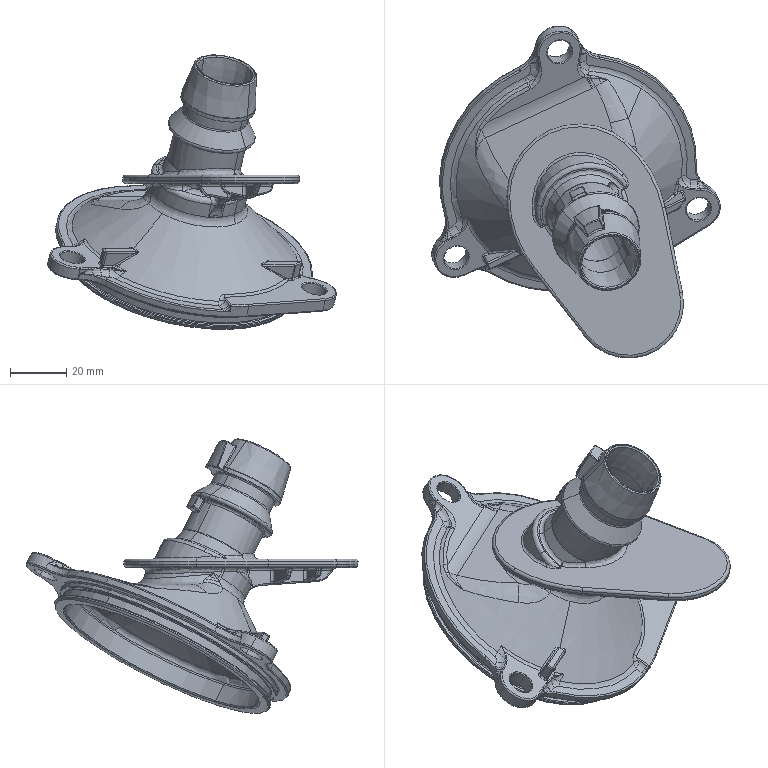Part | SolidWorks | features BaseBody 1 | 1 solid | 669 faces | box 102.773 x 118.28 x 97.783 mm | volume 55614 mm3 | spline 224 | cylinder 165 | torus 155 | plane 63 | cone 43 | sphere 19 | commonest cylinder face diameters 1 x40 2 x37 0.6 x10 3 x6 6 x6 8.9 x6